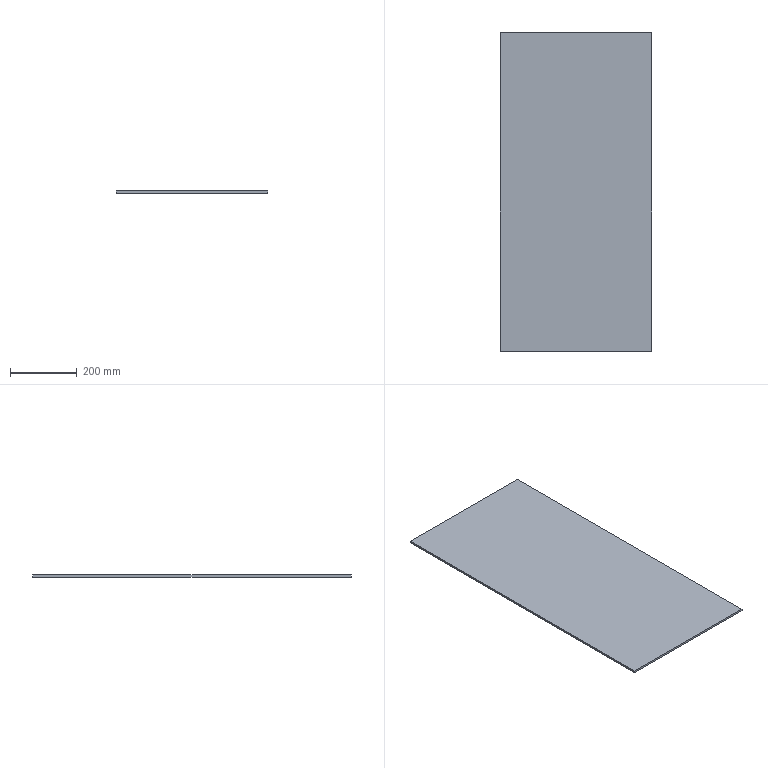Part | SolidWorks | features BaseBody 1 | 1 solid | 6 faces | box 453 x 951 x 6 mm | volume 2584818 mm3 | plane 6
STEP:
#1=CARTESIAN_POINT('',(0.,951.,0.));
#2=VERTEX_POINT('',#1);
#3=CARTESIAN_POINT('',(0.,0.,0.));
#4=VERTEX_POINT('',#3);
#5=CARTESIAN_POINT('',(0.,0.,0.));
#6=DIRECTION('',(0.,-1.,0.));
#7=VECTOR('',#6,1000.);
#8=LINE('',#5,#7);
#9=EDGE_CURVE('',#2,#4,#8,.T.);
#10=ORIENTED_EDGE('',*,*,#9,.F.);
#11=CARTESIAN_POINT('',(453.,951.,0.));
#12=VERTEX_POINT('',#11);
#13=CARTESIAN_POINT('',(0.,951.,0.));
#14=DIRECTION('',(-1.,0.,0.));
#15=VECTOR('',#14,1000.);
#16=LINE('',#13,#15);
#17=EDGE_CURVE('',#12,#2,#16,.T.);
#18=ORIENTED_EDGE('',*,*,#17,.F.);
#19=CARTESIAN_POINT('',(453.,0.,0.));
#20=VERTEX_POINT('',#19);
#21=CARTESIAN_POINT('',(453.,0.,0.));
#22=DIRECTION('',(0.,1.,0.));
#23=VECTOR('',#22,1000.);
#24=LINE('',#21,#23);
#25=EDGE_CURVE('',#20,#12,#24,.T.);
#26=ORIENTED_EDGE('',*,*,#25,.F.);
#27=CARTESIAN_POINT('',(0.,0.,0.));
#28=DIRECTION('',(1.,0.,0.));
#29=VECTOR('',#28,1000.);
#30=LINE('',#27,#29);
#31=EDGE_CURVE('',#4,#20,#30,.T.);
#32=ORIENTED_EDGE('',*,*,#31,.F.);
#33=EDGE_LOOP('',(#10,#18,#26,#32));
#34=FACE_OUTER_BOUND('',#33,.T.);
#35=CARTESIAN_POINT('',(0.,0.,0.));
#36=DIRECTION('',(0.,0.,-1.));
#37=DIRECTION('',(0.,-1.,0.));
#38=AXIS2_PLACEMENT_3D('',#35,#36,#37);
#39=PLANE('',#38);
#40=ADVANCED_FACE('',(#34),#39,.T.);
#41=CARTESIAN_POINT('',(0.,951.,6.));
#42=VERTEX_POINT('',#41);
#43=CARTESIAN_POINT('',(0.,0.,6.));
#44=VERTEX_POINT('',#43);
#45=CARTESIAN_POINT('',(0.,0.,6.));
#46=DIRECTION('',(0.,-1.,0.));
#47=VECTOR('',#46,1000.);
#48=LINE('',#45,#47);
#49=EDGE_CURVE('',#42,#44,#48,.T.);
#50=ORIENTED_EDGE('',*,*,#49,.T.);
#51=CARTESIAN_POINT('',(453.,0.,6.));
#52=VERTEX_POINT('',#51);
#53=CARTESIAN_POINT('',(0.,0.,6.));
#54=DIRECTION('',(1.,0.,0.));
#55=VECTOR('',#54,1000.);
#56=LINE('',#53,#55);
#57=EDGE_CURVE('',#44,#52,#56,.T.);
#58=ORIENTED_EDGE('',*,*,#57,.T.);
#59=CARTESIAN_POINT('',(453.,951.,6.));
#60=VERTEX_POINT('',#59);
#61=CARTESIAN_POINT('',(453.,0.,6.));
#62=DIRECTION('',(0.,1.,0.));
#63=VECTOR('',#62,1000.);
#64=LINE('',#61,#63);
#65=EDGE_CURVE('',#52,#60,#64,.T.);
#66=ORIENTED_EDGE('',*,*,#65,.T.);
#67=CARTESIAN_POINT('',(0.,951.,6.));
#68=DIRECTION('',(-1.,0.,0.));
#69=VECTOR('',#68,1000.);
#70=LINE('',#67,#69);
#71=EDGE_CURVE('',#60,#42,#70,.T.);
#72=ORIENTED_EDGE('',*,*,#71,.T.);
#73=EDGE_LOOP('',(#50,#58,#66,#72));
#74=FACE_OUTER_BOUND('',#73,.T.);
#75=CARTESIAN_POINT('',(0.,0.,6.));
#76=DIRECTION('',(0.,0.,-1.));
#77=DIRECTION('',(0.,-1.,0.));
#78=AXIS2_PLACEMENT_3D('',#75,#76,#77);
#79=PLANE('',#78);
#80=ADVANCED_FACE('',(#74),#79,.F.);
#81=ORIENTED_EDGE('',*,*,#17,.T.);
#82=CARTESIAN_POINT('',(0.,951.,6.));
#83=DIRECTION('',(0.,0.,-1.));
#84=VECTOR('',#83,1000.);
#85=LINE('',#82,#84);
#86=EDGE_CURVE('',#42,#2,#85,.T.);
#87=ORIENTED_EDGE('',*,*,#86,.F.);
#88=ORIENTED_EDGE('',*,*,#71,.F.);
#89=CARTESIAN_POINT('',(453.,951.,6.));
#90=DIRECTION('',(0.,0.,-1.));
#91=VECTOR('',#90,1000.);
#92=LINE('',#89,#91);
#93=EDGE_CURVE('',#60,#12,#92,.T.);
#94=ORIENTED_EDGE('',*,*,#93,.T.);
#95=EDGE_LOOP('',(#81,#87,#88,#94));
#96=FACE_OUTER_BOUND('',#95,.T.);
#97=CARTESIAN_POINT('',(0.,951.,6.));
#98=DIRECTION('',(0.,-1.,0.));
#99=DIRECTION('',(0.,0.,-1.));
#100=AXIS2_PLACEMENT_3D('',#97,#98,#99);
#101=PLANE('',#100);
#102=ADVANCED_FACE('',(#96),#101,.F.);
#103=ORIENTED_EDGE('',*,*,#25,.T.);
#104=ORIENTED_EDGE('',*,*,#93,.F.);
#105=ORIENTED_EDGE('',*,*,#65,.F.);
#106=CARTESIAN_POINT('',(453.,0.,6.));
#107=DIRECTION('',(0.,0.,-1.));
#108=VECTOR('',#107,1000.);
#109=LINE('',#106,#108);
#110=EDGE_CURVE('',#52,#20,#109,.T.);
#111=ORIENTED_EDGE('',*,*,#110,.T.);
#112=EDGE_LOOP('',(#103,#104,#105,#111));
#113=FACE_OUTER_BOUND('',#112,.T.);
#114=CARTESIAN_POINT('',(453.,0.,6.));
#115=DIRECTION('',(-1.,0.,0.));
#116=DIRECTION('',(0.,0.,1.));
#117=AXIS2_PLACEMENT_3D('',#114,#115,#116);
#118=PLANE('',#117);
#119=ADVANCED_FACE('',(#113),#118,.F.);
#120=ORIENTED_EDGE('',*,*,#31,.T.);
#121=ORIENTED_EDGE('',*,*,#110,.F.);
#122=ORIENTED_EDGE('',*,*,#57,.F.);
#123=CARTESIAN_POINT('',(0.,0.,6.));
#124=DIRECTION('',(0.,0.,-1.));
#125=VECTOR('',#124,1000.);
#126=LINE('',#123,#125);
#127=EDGE_CURVE('',#44,#4,#126,.T.);
#128=ORIENTED_EDGE('',*,*,#127,.T.);
#129=EDGE_LOOP('',(#120,#121,#122,#128));
#130=FACE_OUTER_BOUND('',#129,.T.);
#131=CARTESIAN_POINT('',(0.,0.,6.));
#132=DIRECTION('',(0.,1.,0.));
#133=DIRECTION('',(1.,0.,0.));
#134=AXIS2_PLACEMENT_3D('',#131,#132,#133);
#135=PLANE('',#134);
#136=ADVANCED_FACE('',(#130),#135,.F.);
#137=ORIENTED_EDGE('',*,*,#9,.T.);
#138=ORIENTED_EDGE('',*,*,#127,.F.);
#139=ORIENTED_EDGE('',*,*,#49,.F.);
#140=ORIENTED_EDGE('',*,*,#86,.T.);
#141=EDGE_LOOP('',(#137,#138,#139,#140));
#142=FACE_OUTER_BOUND('',#141,.T.);
#143=CARTESIAN_POINT('',(0.,0.,6.));
#144=DIRECTION('',(1.,0.,0.));
#145=DIRECTION('',(0.,1.,0.));
#146=AXIS2_PLACEMENT_3D('',#143,#144,#145);
#147=PLANE('',#146);
#148=ADVANCED_FACE('',(#142),#147,.F.);
#149=CLOSED_SHELL('',(#40,#80,#102,#119,#136,#148));
#150=MANIFOLD_SOLID_BREP('',#149);
#151=CARTESIAN_POINT('',(0.,0.,0.));
#152=DIRECTION('',(0.,0.,1.));
#153=DIRECTION('',(1.,0.,0.));
#154=AXIS2_PLACEMENT_3D('',#151,#152,#153);
#155=(LENGTH_UNIT()NAMED_UNIT(*)SI_UNIT(.MILLI.,.METRE.));
#156=UNCERTAINTY_MEASURE_WITH_UNIT(LENGTH_MEASURE(0.00001),#155,'','');
#157=(NAMED_UNIT(*)PLANE_ANGLE_UNIT()SI_UNIT($,.RADIAN.));
#158=(NAMED_UNIT(*)SI_UNIT($,.STERADIAN.)SOLID_ANGLE_UNIT());
#159=(GEOMETRIC_REPRESENTATION_CONTEXT(3)GLOBAL_UNCERTAINTY_ASSIGNED_CONTEXT((#156))GLOBAL_UNIT_ASSIGNED_CONTEXT((#155,#157,#158))REPRESENTATION_CONTEXT('',''));
#160=ADVANCED_BREP_SHAPE_REPRESENTATION('',(#150,#154),#159);